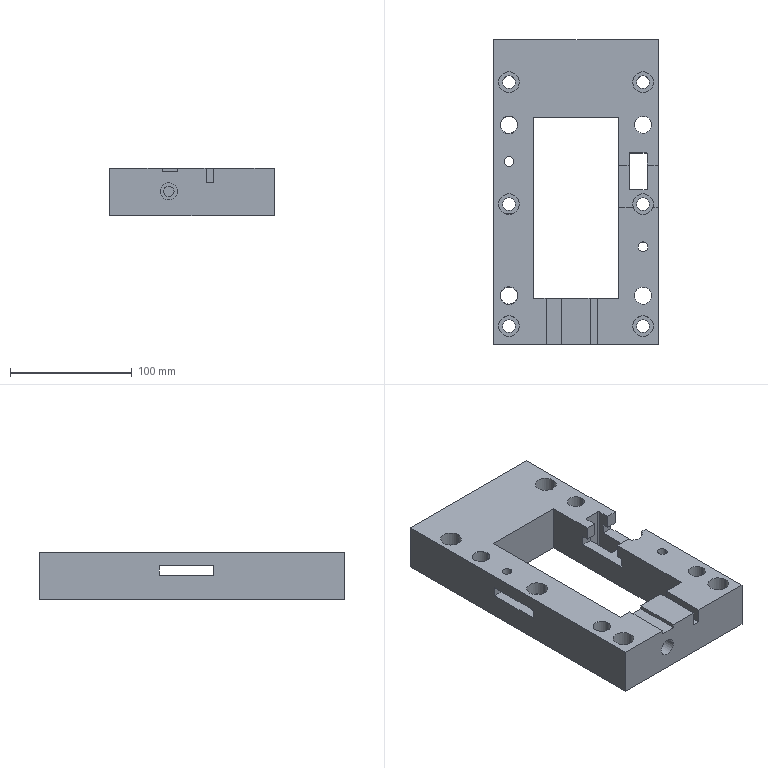Part | STEP file | KHUON BAO DUOI | 1 solid | 100 faces | box 135 x 250 x 39.2 mm | volume 803564 mm3 | plane 47 | cylinder 45 | cone 8 | commonest cylinder face diameters 10.5 x12 17 x12 14 x10 8 x5 2 x4 8.5 x2